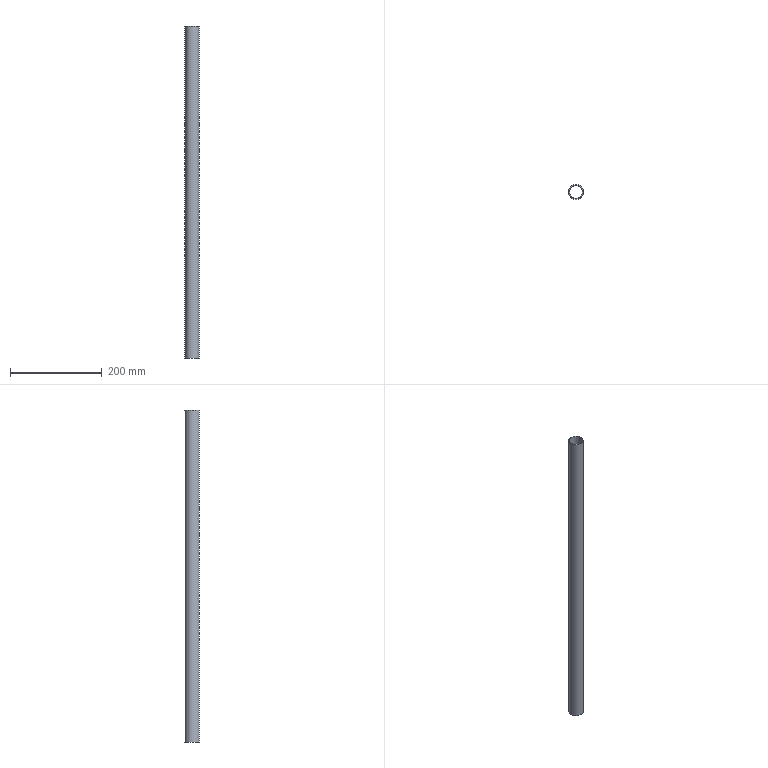Part | STEP file | 7101301 | 1 solid | 4 faces | box 31.8 x 31.8 x 725 mm | volume 103519 mm3 | plane 2 | cylinder 2 | commonest cylinder face diameters 28.8 x1 31.8 x1
STEP:
#1=CARTESIAN_POINT('',(0.,0.,0.));
#2=DIRECTION('',(0.,0.,1.));
#3=DIRECTION('',(1.,0.,0.));
#4=AXIS2_PLACEMENT_3D('',#1,#2,#3);
#5=CARTESIAN_POINT('',(15.9,0.,362.5));
#6=VERTEX_POINT('',#5);
#7=CARTESIAN_POINT('',(0.,0.,362.5));
#8=DIRECTION('',(0.,0.,1.));
#9=DIRECTION('',(1.,0.,0.));
#10=AXIS2_PLACEMENT_3D('',#7,#8,#9);
#11=CIRCLE('',#10,15.9);
#12=CARTESIAN_POINT('',(0.,0.,362.5));
#13=DIRECTION('',(0.,0.,1.));
#14=DIRECTION('',(1.,0.,0.));
#15=AXIS2_PLACEMENT_3D('',#12,#13,#14);
#16=PLANE('',#15);
#17=CARTESIAN_POINT('',(0.,0.));
#18=DIRECTION('',(1.,0.));
#19=AXIS2_PLACEMENT_2D('',#17,#18);
#20=CIRCLE('',#19,15.9);
#21=(GEOMETRIC_REPRESENTATION_CONTEXT(2)PARAMETRIC_REPRESENTATION_CONTEXT()REPRESENTATION_CONTEXT('',''));
#22=DEFINITIONAL_REPRESENTATION('',(#20),#21);
#23=PCURVE('',#16,#22);
#24=CARTESIAN_POINT('',(0.,0.,362.5));
#25=DIRECTION('',(0.,0.,-1.));
#26=DIRECTION('',(-1.,0.,0.));
#27=AXIS2_PLACEMENT_3D('',#24,#25,#26);
#28=CYLINDRICAL_SURFACE('',#27,15.9);
#29=CARTESIAN_POINT('',(9.425,0.));
#30=DIRECTION('',(-1.,0.));
#31=VECTOR('',#30,1.);
#32=LINE('',#29,#31);
#33=(GEOMETRIC_REPRESENTATION_CONTEXT(2)PARAMETRIC_REPRESENTATION_CONTEXT()REPRESENTATION_CONTEXT('',''));
#34=DEFINITIONAL_REPRESENTATION('',(#32),#33);
#35=PCURVE('',#28,#34);
#36=SURFACE_CURVE('',#11,(#23,#35),.PCURVE_S1.);
#37=EDGE_CURVE('',#6,#6,#36,.T.);
#38=ORIENTED_EDGE('',*,*,#37,.T.);
#39=EDGE_LOOP('',(#38));
#40=FACE_BOUND('',#39,.T.);
#41=CARTESIAN_POINT('',(14.4,0.,362.5));
#42=VERTEX_POINT('',#41);
#43=CARTESIAN_POINT('',(0.,0.,362.5));
#44=DIRECTION('',(0.,0.,1.));
#45=DIRECTION('',(1.,0.,0.));
#46=AXIS2_PLACEMENT_3D('',#43,#44,#45);
#47=CIRCLE('',#46,14.4);
#48=CARTESIAN_POINT('',(0.,0.));
#49=DIRECTION('',(1.,0.));
#50=AXIS2_PLACEMENT_2D('',#48,#49);
#51=CIRCLE('',#50,14.4);
#52=(GEOMETRIC_REPRESENTATION_CONTEXT(2)PARAMETRIC_REPRESENTATION_CONTEXT()REPRESENTATION_CONTEXT('',''));
#53=DEFINITIONAL_REPRESENTATION('',(#51),#52);
#54=PCURVE('',#16,#53);
#55=CARTESIAN_POINT('',(0.,0.,362.5));
#56=DIRECTION('',(0.,0.,-1.));
#57=DIRECTION('',(-1.,0.,0.));
#58=AXIS2_PLACEMENT_3D('',#55,#56,#57);
#59=CYLINDRICAL_SURFACE('',#58,14.4);
#60=CARTESIAN_POINT('',(9.425,0.));
#61=DIRECTION('',(-1.,0.));
#62=VECTOR('',#61,1.);
#63=LINE('',#60,#62);
#64=(GEOMETRIC_REPRESENTATION_CONTEXT(2)PARAMETRIC_REPRESENTATION_CONTEXT()REPRESENTATION_CONTEXT('',''));
#65=DEFINITIONAL_REPRESENTATION('',(#63),#64);
#66=PCURVE('',#59,#65);
#67=SURFACE_CURVE('',#47,(#54,#66),.PCURVE_S1.);
#68=EDGE_CURVE('',#42,#42,#67,.T.);
#69=ORIENTED_EDGE('',*,*,#68,.F.);
#70=EDGE_LOOP('',(#69));
#71=FACE_BOUND('',#70,.T.);
#72=ADVANCED_FACE('',(#40,#71),#16,.T.);
#73=CARTESIAN_POINT('',(15.9,0.,-362.5));
#74=VERTEX_POINT('',#73);
#75=CARTESIAN_POINT('',(0.,0.,-362.5));
#76=DIRECTION('',(0.,0.,1.));
#77=DIRECTION('',(1.,0.,0.));
#78=AXIS2_PLACEMENT_3D('',#75,#76,#77);
#79=CIRCLE('',#78,15.9);
#80=CARTESIAN_POINT('',(0.,0.,-362.5));
#81=DIRECTION('',(0.,0.,1.));
#82=DIRECTION('',(1.,0.,0.));
#83=AXIS2_PLACEMENT_3D('',#80,#81,#82);
#84=PLANE('',#83);
#85=CARTESIAN_POINT('',(0.,0.));
#86=DIRECTION('',(1.,0.));
#87=AXIS2_PLACEMENT_2D('',#85,#86);
#88=CIRCLE('',#87,15.9);
#89=(GEOMETRIC_REPRESENTATION_CONTEXT(2)PARAMETRIC_REPRESENTATION_CONTEXT()REPRESENTATION_CONTEXT('',''));
#90=DEFINITIONAL_REPRESENTATION('',(#88),#89);
#91=PCURVE('',#84,#90);
#92=CARTESIAN_POINT('',(9.425,725.));
#93=DIRECTION('',(-1.,0.));
#94=VECTOR('',#93,1.);
#95=LINE('',#92,#94);
#96=(GEOMETRIC_REPRESENTATION_CONTEXT(2)PARAMETRIC_REPRESENTATION_CONTEXT()REPRESENTATION_CONTEXT('',''));
#97=DEFINITIONAL_REPRESENTATION('',(#95),#96);
#98=PCURVE('',#28,#97);
#99=SURFACE_CURVE('',#79,(#91,#98),.PCURVE_S1.);
#100=EDGE_CURVE('',#74,#74,#99,.T.);
#101=ORIENTED_EDGE('',*,*,#100,.F.);
#102=EDGE_LOOP('',(#101));
#103=FACE_BOUND('',#102,.T.);
#104=CARTESIAN_POINT('',(14.4,0.,-362.5));
#105=VERTEX_POINT('',#104);
#106=CARTESIAN_POINT('',(0.,0.,-362.5));
#107=DIRECTION('',(0.,0.,1.));
#108=DIRECTION('',(1.,0.,0.));
#109=AXIS2_PLACEMENT_3D('',#106,#107,#108);
#110=CIRCLE('',#109,14.4);
#111=CARTESIAN_POINT('',(0.,0.));
#112=DIRECTION('',(1.,0.));
#113=AXIS2_PLACEMENT_2D('',#111,#112);
#114=CIRCLE('',#113,14.4);
#115=(GEOMETRIC_REPRESENTATION_CONTEXT(2)PARAMETRIC_REPRESENTATION_CONTEXT()REPRESENTATION_CONTEXT('',''));
#116=DEFINITIONAL_REPRESENTATION('',(#114),#115);
#117=PCURVE('',#84,#116);
#118=CARTESIAN_POINT('',(9.425,725.));
#119=DIRECTION('',(-1.,0.));
#120=VECTOR('',#119,1.);
#121=LINE('',#118,#120);
#122=(GEOMETRIC_REPRESENTATION_CONTEXT(2)PARAMETRIC_REPRESENTATION_CONTEXT()REPRESENTATION_CONTEXT('',''));
#123=DEFINITIONAL_REPRESENTATION('',(#121),#122);
#124=PCURVE('',#59,#123);
#125=SURFACE_CURVE('',#110,(#117,#124),.PCURVE_S1.);
#126=EDGE_CURVE('',#105,#105,#125,.T.);
#127=ORIENTED_EDGE('',*,*,#126,.T.);
#128=EDGE_LOOP('',(#127));
#129=FACE_BOUND('',#128,.T.);
#130=ADVANCED_FACE('',(#103,#129),#84,.F.);
#131=ORIENTED_EDGE('',*,*,#37,.F.);
#132=CARTESIAN_POINT('',(15.9,0.,362.5));
#133=CARTESIAN_POINT('',(15.9,0.,-362.5));
#134=B_SPLINE_CURVE_WITH_KNOTS('',1,(#132,#133),.UNSPECIFIED.,.F.,.F.,(2,2),(0.,725.),.PIECEWISE_BEZIER_KNOTS.);
#135=CARTESIAN_POINT('',(9.425,0.));
#136=DIRECTION('',(0.,1.));
#137=VECTOR('',#136,1.);
#138=LINE('',#135,#137);
#139=(GEOMETRIC_REPRESENTATION_CONTEXT(2)PARAMETRIC_REPRESENTATION_CONTEXT()REPRESENTATION_CONTEXT('',''));
#140=DEFINITIONAL_REPRESENTATION('',(#138),#139);
#141=PCURVE('',#28,#140);
#142=CARTESIAN_POINT('',(3.142,0.));
#143=DIRECTION('',(0.,1.));
#144=VECTOR('',#143,1.);
#145=LINE('',#142,#144);
#146=(GEOMETRIC_REPRESENTATION_CONTEXT(2)PARAMETRIC_REPRESENTATION_CONTEXT()REPRESENTATION_CONTEXT('',''));
#147=DEFINITIONAL_REPRESENTATION('',(#145),#146);
#148=PCURVE('',#28,#147);
#149=SEAM_CURVE('',#134,(#141,#148),.PCURVE_S1.);
#150=EDGE_CURVE('',#6,#74,#149,.T.);
#151=ORIENTED_EDGE('',*,*,#150,.T.);
#152=ORIENTED_EDGE('',*,*,#100,.T.);
#153=ORIENTED_EDGE('',*,*,#150,.F.);
#154=EDGE_LOOP('',(#131,#151,#152,#153));
#155=FACE_BOUND('',#154,.T.);
#156=ADVANCED_FACE('',(#155),#28,.T.);
#157=ORIENTED_EDGE('',*,*,#68,.F.);
#158=CARTESIAN_POINT('',(14.4,0.,362.5));
#159=CARTESIAN_POINT('',(14.4,0.,-362.5));
#160=B_SPLINE_CURVE_WITH_KNOTS('',1,(#158,#159),.UNSPECIFIED.,.F.,.F.,(2,2),(0.,725.),.PIECEWISE_BEZIER_KNOTS.);
#161=CARTESIAN_POINT('',(9.425,0.));
#162=DIRECTION('',(0.,1.));
#163=VECTOR('',#162,1.);
#164=LINE('',#161,#163);
#165=(GEOMETRIC_REPRESENTATION_CONTEXT(2)PARAMETRIC_REPRESENTATION_CONTEXT()REPRESENTATION_CONTEXT('',''));
#166=DEFINITIONAL_REPRESENTATION('',(#164),#165);
#167=PCURVE('',#59,#166);
#168=CARTESIAN_POINT('',(3.142,0.));
#169=DIRECTION('',(0.,1.));
#170=VECTOR('',#169,1.);
#171=LINE('',#168,#170);
#172=(GEOMETRIC_REPRESENTATION_CONTEXT(2)PARAMETRIC_REPRESENTATION_CONTEXT()REPRESENTATION_CONTEXT('',''));
#173=DEFINITIONAL_REPRESENTATION('',(#171),#172);
#174=PCURVE('',#59,#173);
#175=SEAM_CURVE('',#160,(#167,#174),.PCURVE_S1.);
#176=EDGE_CURVE('',#42,#105,#175,.T.);
#177=ORIENTED_EDGE('',*,*,#176,.T.);
#178=ORIENTED_EDGE('',*,*,#126,.T.);
#179=ORIENTED_EDGE('',*,*,#176,.F.);
#180=EDGE_LOOP('',(#157,#177,#178,#179));
#181=FACE_BOUND('',#180,.F.);
#182=ADVANCED_FACE('',(#181),#59,.F.);
#183=CLOSED_SHELL('',(#72,#130,#156,#182));
#184=MANIFOLD_SOLID_BREP('',#183);
#185=(LENGTH_UNIT()NAMED_UNIT(*)SI_UNIT(.MILLI.,.METRE.));
#186=UNCERTAINTY_MEASURE_WITH_UNIT(LENGTH_MEASURE(0.00001),#185,'','');
#187=(NAMED_UNIT(*)PLANE_ANGLE_UNIT()SI_UNIT($,.RADIAN.));
#188=(NAMED_UNIT(*)SI_UNIT($,.STERADIAN.)SOLID_ANGLE_UNIT());
#189=(GEOMETRIC_REPRESENTATION_CONTEXT(3)GLOBAL_UNCERTAINTY_ASSIGNED_CONTEXT((#186))GLOBAL_UNIT_ASSIGNED_CONTEXT((#185,#187,#188))REPRESENTATION_CONTEXT('',''));
#190=ADVANCED_BREP_SHAPE_REPRESENTATION('',(#4,#184),#189);